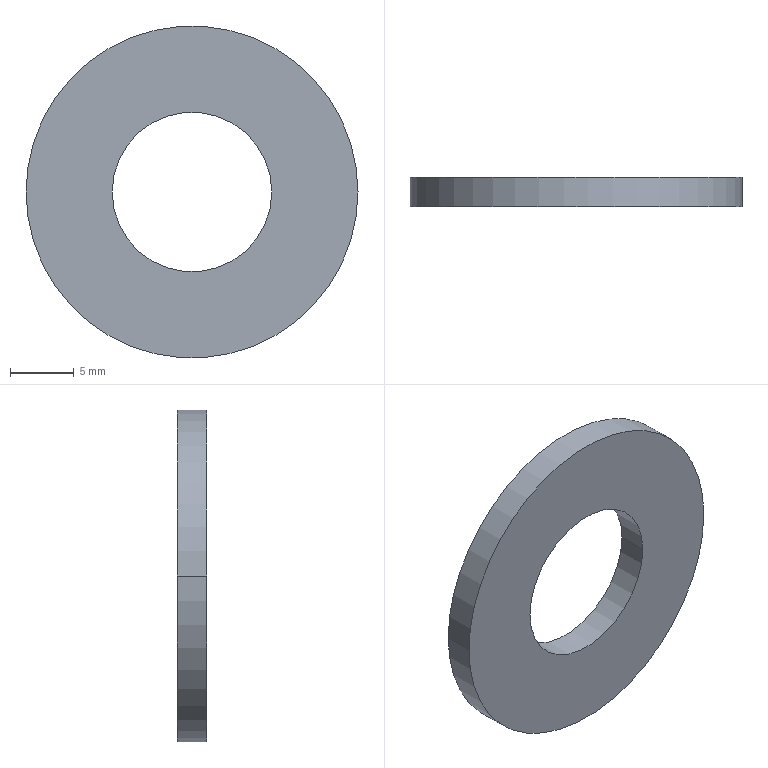Part | STEP file | ZZ21-M12 | 1 solid | 6 faces | box 26 x 2.3 x 26 mm | volume 938.885 mm3 | cylinder 4 | plane 2 | commonest cylinder face diameters 12.5 x2 26 x2
STEP:
#1=CARTESIAN_POINT('',(0.,0.,0.));
#2=DIRECTION('',(0.,0.,1.));
#3=DIRECTION('',(1.,0.,0.));
#4=AXIS2_PLACEMENT_3D('',#1,#2,#3);
#5=CARTESIAN_POINT('',(-6.25,0.,0.));
#6=VERTEX_POINT('',#5);
#7=CARTESIAN_POINT('',(-6.25,2.3,0.));
#8=VERTEX_POINT('',#7);
#9=CARTESIAN_POINT('',(-6.25,0.,0.));
#10=DIRECTION('',(0.,1.,0.));
#11=VECTOR('',#10,1.);
#12=LINE('',#9,#11);
#13=CARTESIAN_POINT('',(0.,0.,0.));
#14=DIRECTION('',(0.,1.,0.));
#15=DIRECTION('',(-1.,0.,0.));
#16=AXIS2_PLACEMENT_3D('',#13,#14,#15);
#17=CYLINDRICAL_SURFACE('',#16,6.25);
#18=CARTESIAN_POINT('',(6.283,0.));
#19=DIRECTION('',(0.,1.));
#20=VECTOR('',#19,1.);
#21=LINE('',#18,#20);
#22=(GEOMETRIC_REPRESENTATION_CONTEXT(2)PARAMETRIC_REPRESENTATION_CONTEXT()REPRESENTATION_CONTEXT('',''));
#23=DEFINITIONAL_REPRESENTATION('',(#21),#22);
#24=PCURVE('',#17,#23);
#25=CARTESIAN_POINT('',(0.,0.,0.));
#26=DIRECTION('',(0.,1.,0.));
#27=DIRECTION('',(-1.,0.,0.));
#28=AXIS2_PLACEMENT_3D('',#25,#26,#27);
#29=CYLINDRICAL_SURFACE('',#28,6.25);
#30=CARTESIAN_POINT('',(0.,0.));
#31=DIRECTION('',(0.,1.));
#32=VECTOR('',#31,1.);
#33=LINE('',#30,#32);
#34=(GEOMETRIC_REPRESENTATION_CONTEXT(2)PARAMETRIC_REPRESENTATION_CONTEXT()REPRESENTATION_CONTEXT('',''));
#35=DEFINITIONAL_REPRESENTATION('',(#33),#34);
#36=PCURVE('',#29,#35);
#37=SURFACE_CURVE('',#12,(#24,#36),.PCURVE_S1.);
#38=EDGE_CURVE('',#6,#8,#37,.T.);
#39=ORIENTED_EDGE('',*,*,#38,.T.);
#40=CARTESIAN_POINT('',(6.25,2.3,0.));
#41=VERTEX_POINT('',#40);
#42=CARTESIAN_POINT('',(0.,2.3,0.));
#43=DIRECTION('',(0.,-1.,0.));
#44=DIRECTION('',(1.,0.,0.));
#45=AXIS2_PLACEMENT_3D('',#42,#43,#44);
#46=CIRCLE('',#45,6.25);
#47=CARTESIAN_POINT('',(9.425,2.3));
#48=DIRECTION('',(-1.,0.));
#49=VECTOR('',#48,1.);
#50=LINE('',#47,#49);
#51=(GEOMETRIC_REPRESENTATION_CONTEXT(2)PARAMETRIC_REPRESENTATION_CONTEXT()REPRESENTATION_CONTEXT('',''));
#52=DEFINITIONAL_REPRESENTATION('',(#50),#51);
#53=PCURVE('',#17,#52);
#54=CARTESIAN_POINT('',(0.,2.3,0.));
#55=DIRECTION('',(0.,1.,0.));
#56=DIRECTION('',(-1.,0.,0.));
#57=AXIS2_PLACEMENT_3D('',#54,#55,#56);
#58=PLANE('',#57);
#59=CARTESIAN_POINT('',(-6.25,0.));
#60=CARTESIAN_POINT('',(-6.25,10.825));
#61=CARTESIAN_POINT('',(3.125,5.413));
#62=CARTESIAN_POINT('',(12.5,0.));
#63=CARTESIAN_POINT('',(3.125,-5.413));
#64=CARTESIAN_POINT('',(-6.25,-10.825));
#65=CARTESIAN_POINT('',(-6.25,0.));
#66=(BOUNDED_CURVE()B_SPLINE_CURVE(2,(#59,#60,#61,#62,#63,#64,#65),.UNSPECIFIED.,.T.,.F.)B_SPLINE_CURVE_WITH_KNOTS((1,2,2,2,2,1),(-2.094,0.,2.094,4.189,6.283,8.378),.UNSPECIFIED.)CURVE()GEOMETRIC_REPRESENTATION_ITEM()RATIONAL_B_SPLINE_CURVE((1.,0.5,1.,0.5,1.,0.5,1.))REPRESENTATION_ITEM(''));
#67=(GEOMETRIC_REPRESENTATION_CONTEXT(2)PARAMETRIC_REPRESENTATION_CONTEXT()REPRESENTATION_CONTEXT('',''));
#68=DEFINITIONAL_REPRESENTATION('',(#66),#67);
#69=PCURVE('',#58,#68);
#70=SURFACE_CURVE('',#46,(#53,#69),.PCURVE_S1.);
#71=EDGE_CURVE('',#8,#41,#70,.T.);
#72=ORIENTED_EDGE('',*,*,#71,.T.);
#73=CARTESIAN_POINT('',(6.25,0.,0.));
#74=VERTEX_POINT('',#73);
#75=CARTESIAN_POINT('',(6.25,0.,0.));
#76=DIRECTION('',(0.,1.,0.));
#77=VECTOR('',#76,1.);
#78=LINE('',#75,#77);
#79=CARTESIAN_POINT('',(3.142,0.));
#80=DIRECTION('',(0.,1.));
#81=VECTOR('',#80,1.);
#82=LINE('',#79,#81);
#83=(GEOMETRIC_REPRESENTATION_CONTEXT(2)PARAMETRIC_REPRESENTATION_CONTEXT()REPRESENTATION_CONTEXT('',''));
#84=DEFINITIONAL_REPRESENTATION('',(#82),#83);
#85=PCURVE('',#17,#84);
#86=CARTESIAN_POINT('',(3.142,0.));
#87=DIRECTION('',(0.,1.));
#88=VECTOR('',#87,1.);
#89=LINE('',#86,#88);
#90=(GEOMETRIC_REPRESENTATION_CONTEXT(2)PARAMETRIC_REPRESENTATION_CONTEXT()REPRESENTATION_CONTEXT('',''));
#91=DEFINITIONAL_REPRESENTATION('',(#89),#90);
#92=PCURVE('',#29,#91);
#93=SURFACE_CURVE('',#78,(#85,#92),.PCURVE_S1.);
#94=EDGE_CURVE('',#74,#41,#93,.T.);
#95=ORIENTED_EDGE('',*,*,#94,.F.);
#96=CARTESIAN_POINT('',(0.,0.,0.));
#97=DIRECTION('',(0.,1.,0.));
#98=DIRECTION('',(-1.,0.,0.));
#99=AXIS2_PLACEMENT_3D('',#96,#97,#98);
#100=CIRCLE('',#99,6.25);
#101=CARTESIAN_POINT('',(0.,0.));
#102=DIRECTION('',(1.,0.));
#103=VECTOR('',#102,1.);
#104=LINE('',#101,#103);
#105=(GEOMETRIC_REPRESENTATION_CONTEXT(2)PARAMETRIC_REPRESENTATION_CONTEXT()REPRESENTATION_CONTEXT('',''));
#106=DEFINITIONAL_REPRESENTATION('',(#104),#105);
#107=PCURVE('',#17,#106);
#108=CARTESIAN_POINT('',(0.,0.,0.));
#109=DIRECTION('',(0.,-1.,0.));
#110=DIRECTION('',(1.,0.,0.));
#111=AXIS2_PLACEMENT_3D('',#108,#109,#110);
#112=PLANE('',#111);
#113=CARTESIAN_POINT('',(-6.25,0.));
#114=CARTESIAN_POINT('',(-6.25,10.825));
#115=CARTESIAN_POINT('',(3.125,5.413));
#116=CARTESIAN_POINT('',(12.5,0.));
#117=CARTESIAN_POINT('',(3.125,-5.413));
#118=CARTESIAN_POINT('',(-6.25,-10.825));
#119=CARTESIAN_POINT('',(-6.25,0.));
#120=(BOUNDED_CURVE()B_SPLINE_CURVE(2,(#113,#114,#115,#116,#117,#118,#119),.UNSPECIFIED.,.T.,.F.)B_SPLINE_CURVE_WITH_KNOTS((1,2,2,2,2,1),(-2.094,0.,2.094,4.189,6.283,8.378),.UNSPECIFIED.)CURVE()GEOMETRIC_REPRESENTATION_ITEM()RATIONAL_B_SPLINE_CURVE((1.,0.5,1.,0.5,1.,0.5,1.))REPRESENTATION_ITEM(''));
#121=(GEOMETRIC_REPRESENTATION_CONTEXT(2)PARAMETRIC_REPRESENTATION_CONTEXT()REPRESENTATION_CONTEXT('',''));
#122=DEFINITIONAL_REPRESENTATION('',(#120),#121);
#123=PCURVE('',#112,#122);
#124=SURFACE_CURVE('',#100,(#107,#123),.PCURVE_S1.);
#125=EDGE_CURVE('',#74,#6,#124,.T.);
#126=ORIENTED_EDGE('',*,*,#125,.T.);
#127=EDGE_LOOP('',(#39,#72,#95,#126));
#128=FACE_BOUND('',#127,.F.);
#129=ADVANCED_FACE('',(#128),#17,.F.);
#130=CARTESIAN_POINT('',(-13.,0.,0.));
#131=VERTEX_POINT('',#130);
#132=CARTESIAN_POINT('',(13.,0.,0.));
#133=VERTEX_POINT('',#132);
#134=CARTESIAN_POINT('',(0.,0.,0.));
#135=DIRECTION('',(0.,1.,0.));
#136=DIRECTION('',(-1.,0.,0.));
#137=AXIS2_PLACEMENT_3D('',#134,#135,#136);
#138=CIRCLE('',#137,13.);
#139=CARTESIAN_POINT('',(0.,0.,0.));
#140=DIRECTION('',(0.,1.,0.));
#141=DIRECTION('',(-1.,0.,0.));
#142=AXIS2_PLACEMENT_3D('',#139,#140,#141);
#143=CYLINDRICAL_SURFACE('',#142,13.);
#144=CARTESIAN_POINT('',(0.,0.));
#145=DIRECTION('',(1.,0.));
#146=VECTOR('',#145,1.);
#147=LINE('',#144,#146);
#148=(GEOMETRIC_REPRESENTATION_CONTEXT(2)PARAMETRIC_REPRESENTATION_CONTEXT()REPRESENTATION_CONTEXT('',''));
#149=DEFINITIONAL_REPRESENTATION('',(#147),#148);
#150=PCURVE('',#143,#149);
#151=CARTESIAN_POINT('',(-13.,0.));
#152=CARTESIAN_POINT('',(-13.,22.517));
#153=CARTESIAN_POINT('',(6.5,11.258));
#154=CARTESIAN_POINT('',(26.,0.));
#155=CARTESIAN_POINT('',(6.5,-11.258));
#156=CARTESIAN_POINT('',(-13.,-22.517));
#157=CARTESIAN_POINT('',(-13.,0.));
#158=(BOUNDED_CURVE()B_SPLINE_CURVE(2,(#151,#152,#153,#154,#155,#156,#157),.UNSPECIFIED.,.T.,.F.)B_SPLINE_CURVE_WITH_KNOTS((1,2,2,2,2,1),(-2.094,0.,2.094,4.189,6.283,8.378),.UNSPECIFIED.)CURVE()GEOMETRIC_REPRESENTATION_ITEM()RATIONAL_B_SPLINE_CURVE((1.,0.5,1.,0.5,1.,0.5,1.))REPRESENTATION_ITEM(''));
#159=(GEOMETRIC_REPRESENTATION_CONTEXT(2)PARAMETRIC_REPRESENTATION_CONTEXT()REPRESENTATION_CONTEXT('',''));
#160=DEFINITIONAL_REPRESENTATION('',(#158),#159);
#161=PCURVE('',#112,#160);
#162=SURFACE_CURVE('',#138,(#150,#161),.PCURVE_S1.);
#163=EDGE_CURVE('',#131,#133,#162,.T.);
#164=ORIENTED_EDGE('',*,*,#163,.T.);
#165=CARTESIAN_POINT('',(13.,2.3,0.));
#166=VERTEX_POINT('',#165);
#167=CARTESIAN_POINT('',(13.,0.,0.));
#168=DIRECTION('',(0.,1.,0.));
#169=VECTOR('',#168,1.);
#170=LINE('',#167,#169);
#171=CARTESIAN_POINT('',(3.142,0.));
#172=DIRECTION('',(0.,1.));
#173=VECTOR('',#172,1.);
#174=LINE('',#171,#173);
#175=(GEOMETRIC_REPRESENTATION_CONTEXT(2)PARAMETRIC_REPRESENTATION_CONTEXT()REPRESENTATION_CONTEXT('',''));
#176=DEFINITIONAL_REPRESENTATION('',(#174),#175);
#177=PCURVE('',#143,#176);
#178=CARTESIAN_POINT('',(0.,0.,0.));
#179=DIRECTION('',(0.,1.,0.));
#180=DIRECTION('',(-1.,0.,0.));
#181=AXIS2_PLACEMENT_3D('',#178,#179,#180);
#182=CYLINDRICAL_SURFACE('',#181,13.);
#183=CARTESIAN_POINT('',(3.142,0.));
#184=DIRECTION('',(0.,1.));
#185=VECTOR('',#184,1.);
#186=LINE('',#183,#185);
#187=(GEOMETRIC_REPRESENTATION_CONTEXT(2)PARAMETRIC_REPRESENTATION_CONTEXT()REPRESENTATION_CONTEXT('',''));
#188=DEFINITIONAL_REPRESENTATION('',(#186),#187);
#189=PCURVE('',#182,#188);
#190=SURFACE_CURVE('',#170,(#177,#189),.PCURVE_S1.);
#191=EDGE_CURVE('',#133,#166,#190,.T.);
#192=ORIENTED_EDGE('',*,*,#191,.T.);
#193=CARTESIAN_POINT('',(-13.,2.3,0.));
#194=VERTEX_POINT('',#193);
#195=CARTESIAN_POINT('',(0.,2.3,0.));
#196=DIRECTION('',(0.,-1.,0.));
#197=DIRECTION('',(1.,0.,0.));
#198=AXIS2_PLACEMENT_3D('',#195,#196,#197);
#199=CIRCLE('',#198,13.);
#200=CARTESIAN_POINT('',(3.142,2.3));
#201=DIRECTION('',(-1.,0.));
#202=VECTOR('',#201,1.);
#203=LINE('',#200,#202);
#204=(GEOMETRIC_REPRESENTATION_CONTEXT(2)PARAMETRIC_REPRESENTATION_CONTEXT()REPRESENTATION_CONTEXT('',''));
#205=DEFINITIONAL_REPRESENTATION('',(#203),#204);
#206=PCURVE('',#143,#205);
#207=CARTESIAN_POINT('',(-13.,0.));
#208=CARTESIAN_POINT('',(-13.,22.517));
#209=CARTESIAN_POINT('',(6.5,11.258));
#210=CARTESIAN_POINT('',(26.,0.));
#211=CARTESIAN_POINT('',(6.5,-11.258));
#212=CARTESIAN_POINT('',(-13.,-22.517));
#213=CARTESIAN_POINT('',(-13.,0.));
#214=(BOUNDED_CURVE()B_SPLINE_CURVE(2,(#207,#208,#209,#210,#211,#212,#213),.UNSPECIFIED.,.T.,.F.)B_SPLINE_CURVE_WITH_KNOTS((1,2,2,2,2,1),(-2.094,0.,2.094,4.189,6.283,8.378),.UNSPECIFIED.)CURVE()GEOMETRIC_REPRESENTATION_ITEM()RATIONAL_B_SPLINE_CURVE((1.,0.5,1.,0.5,1.,0.5,1.))REPRESENTATION_ITEM(''));
#215=(GEOMETRIC_REPRESENTATION_CONTEXT(2)PARAMETRIC_REPRESENTATION_CONTEXT()REPRESENTATION_CONTEXT('',''));
#216=DEFINITIONAL_REPRESENTATION('',(#214),#215);
#217=PCURVE('',#58,#216);
#218=SURFACE_CURVE('',#199,(#206,#217),.PCURVE_S1.);
#219=EDGE_CURVE('',#166,#194,#218,.T.);
#220=ORIENTED_EDGE('',*,*,#219,.T.);
#221=CARTESIAN_POINT('',(-13.,0.,0.));
#222=DIRECTION('',(0.,1.,0.));
#223=VECTOR('',#222,1.);
#224=LINE('',#221,#223);
#225=CARTESIAN_POINT('',(0.,0.));
#226=DIRECTION('',(0.,1.));
#227=VECTOR('',#226,1.);
#228=LINE('',#225,#227);
#229=(GEOMETRIC_REPRESENTATION_CONTEXT(2)PARAMETRIC_REPRESENTATION_CONTEXT()REPRESENTATION_CONTEXT('',''));
#230=DEFINITIONAL_REPRESENTATION('',(#228),#229);
#231=PCURVE('',#143,#230);
#232=CARTESIAN_POINT('',(6.283,0.));
#233=DIRECTION('',(0.,1.));
#234=VECTOR('',#233,1.);
#235=LINE('',#232,#234);
#236=(GEOMETRIC_REPRESENTATION_CONTEXT(2)PARAMETRIC_REPRESENTATION_CONTEXT()REPRESENTATION_CONTEXT('',''));
#237=DEFINITIONAL_REPRESENTATION('',(#235),#236);
#238=PCURVE('',#182,#237);
#239=SURFACE_CURVE('',#224,(#231,#238),.PCURVE_S1.);
#240=EDGE_CURVE('',#131,#194,#239,.T.);
#241=ORIENTED_EDGE('',*,*,#240,.F.);
#242=EDGE_LOOP('',(#164,#192,#220,#241));
#243=FACE_BOUND('',#242,.T.);
#244=ADVANCED_FACE('',(#243),#143,.T.);
#245=ORIENTED_EDGE('',*,*,#71,.T.);
#246=CARTESIAN_POINT('',(0.,2.3,0.));
#247=DIRECTION('',(0.,-1.,0.));
#248=DIRECTION('',(1.,0.,0.));
#249=AXIS2_PLACEMENT_3D('',#246,#247,#248);
#250=CIRCLE('',#249,6.25);
#251=CARTESIAN_POINT('',(-6.25,0.));
#252=CARTESIAN_POINT('',(-6.25,10.825));
#253=CARTESIAN_POINT('',(3.125,5.413));
#254=CARTESIAN_POINT('',(12.5,0.));
#255=CARTESIAN_POINT('',(3.125,-5.413));
#256=CARTESIAN_POINT('',(-6.25,-10.825));
#257=CARTESIAN_POINT('',(-6.25,0.));
#258=(BOUNDED_CURVE()B_SPLINE_CURVE(2,(#251,#252,#253,#254,#255,#256,#257),.UNSPECIFIED.,.T.,.F.)B_SPLINE_CURVE_WITH_KNOTS((1,2,2,2,2,1),(-2.094,0.,2.094,4.189,6.283,8.378),.UNSPECIFIED.)CURVE()GEOMETRIC_REPRESENTATION_ITEM()RATIONAL_B_SPLINE_CURVE((1.,0.5,1.,0.5,1.,0.5,1.))REPRESENTATION_ITEM(''));
#259=(GEOMETRIC_REPRESENTATION_CONTEXT(2)PARAMETRIC_REPRESENTATION_CONTEXT()REPRESENTATION_CONTEXT('',''));
#260=DEFINITIONAL_REPRESENTATION('',(#258),#259);
#261=PCURVE('',#58,#260);
#262=CARTESIAN_POINT('',(3.142,2.3));
#263=DIRECTION('',(-1.,0.));
#264=VECTOR('',#263,1.);
#265=LINE('',#262,#264);
#266=(GEOMETRIC_REPRESENTATION_CONTEXT(2)PARAMETRIC_REPRESENTATION_CONTEXT()REPRESENTATION_CONTEXT('',''));
#267=DEFINITIONAL_REPRESENTATION('',(#265),#266);
#268=PCURVE('',#29,#267);
#269=SURFACE_CURVE('',#250,(#261,#268),.PCURVE_S1.);
#270=EDGE_CURVE('',#41,#8,#269,.T.);
#271=ORIENTED_EDGE('',*,*,#270,.T.);
#272=EDGE_LOOP('',(#245,#271));
#273=FACE_BOUND('',#272,.T.);
#274=CARTESIAN_POINT('',(0.,2.3,0.));
#275=DIRECTION('',(0.,-1.,0.));
#276=DIRECTION('',(1.,0.,0.));
#277=AXIS2_PLACEMENT_3D('',#274,#275,#276);
#278=CIRCLE('',#277,13.);
#279=CARTESIAN_POINT('',(-13.,0.));
#280=CARTESIAN_POINT('',(-13.,22.517));
#281=CARTESIAN_POINT('',(6.5,11.258));
#282=CARTESIAN_POINT('',(26.,0.));
#283=CARTESIAN_POINT('',(6.5,-11.258));
#284=CARTESIAN_POINT('',(-13.,-22.517));
#285=CARTESIAN_POINT('',(-13.,0.));
#286=(BOUNDED_CURVE()B_SPLINE_CURVE(2,(#279,#280,#281,#282,#283,#284,#285),.UNSPECIFIED.,.T.,.F.)B_SPLINE_CURVE_WITH_KNOTS((1,2,2,2,2,1),(-2.094,0.,2.094,4.189,6.283,8.378),.UNSPECIFIED.)CURVE()GEOMETRIC_REPRESENTATION_ITEM()RATIONAL_B_SPLINE_CURVE((1.,0.5,1.,0.5,1.,0.5,1.))REPRESENTATION_ITEM(''));
#287=(GEOMETRIC_REPRESENTATION_CONTEXT(2)PARAMETRIC_REPRESENTATION_CONTEXT()REPRESENTATION_CONTEXT('',''));
#288=DEFINITIONAL_REPRESENTATION('',(#286),#287);
#289=PCURVE('',#58,#288);
#290=CARTESIAN_POINT('',(9.425,2.3));
#291=DIRECTION('',(-1.,0.));
#292=VECTOR('',#291,1.);
#293=LINE('',#290,#292);
#294=(GEOMETRIC_REPRESENTATION_CONTEXT(2)PARAMETRIC_REPRESENTATION_CONTEXT()REPRESENTATION_CONTEXT('',''));
#295=DEFINITIONAL_REPRESENTATION('',(#293),#294);
#296=PCURVE('',#182,#295);
#297=SURFACE_CURVE('',#278,(#289,#296),.PCURVE_S1.);
#298=EDGE_CURVE('',#194,#166,#297,.T.);
#299=ORIENTED_EDGE('',*,*,#298,.F.);
#300=ORIENTED_EDGE('',*,*,#219,.F.);
#301=EDGE_LOOP('',(#299,#300));
#302=FACE_BOUND('',#301,.T.);
#303=ADVANCED_FACE('',(#273,#302),#58,.T.);
#304=CARTESIAN_POINT('',(0.,0.,0.));
#305=DIRECTION('',(0.,1.,0.));
#306=DIRECTION('',(-1.,0.,0.));
#307=AXIS2_PLACEMENT_3D('',#304,#305,#306);
#308=CIRCLE('',#307,6.25);
#309=CARTESIAN_POINT('',(-6.25,0.));
#310=CARTESIAN_POINT('',(-6.25,10.825));
#311=CARTESIAN_POINT('',(3.125,5.413));
#312=CARTESIAN_POINT('',(12.5,0.));
#313=CARTESIAN_POINT('',(3.125,-5.413));
#314=CARTESIAN_POINT('',(-6.25,-10.825));
#315=CARTESIAN_POINT('',(-6.25,0.));
#316=(BOUNDED_CURVE()B_SPLINE_CURVE(2,(#309,#310,#311,#312,#313,#314,#315),.UNSPECIFIED.,.T.,.F.)B_SPLINE_CURVE_WITH_KNOTS((1,2,2,2,2,1),(-2.094,0.,2.094,4.189,6.283,8.378),.UNSPECIFIED.)CURVE()GEOMETRIC_REPRESENTATION_ITEM()RATIONAL_B_SPLINE_CURVE((1.,0.5,1.,0.5,1.,0.5,1.))REPRESENTATION_ITEM(''));
#317=(GEOMETRIC_REPRESENTATION_CONTEXT(2)PARAMETRIC_REPRESENTATION_CONTEXT()REPRESENTATION_CONTEXT('',''));
#318=DEFINITIONAL_REPRESENTATION('',(#316),#317);
#319=PCURVE('',#112,#318);
#320=CARTESIAN_POINT('',(0.,0.));
#321=DIRECTION('',(1.,0.));
#322=VECTOR('',#321,1.);
#323=LINE('',#320,#322);
#324=(GEOMETRIC_REPRESENTATION_CONTEXT(2)PARAMETRIC_REPRESENTATION_CONTEXT()REPRESENTATION_CONTEXT('',''));
#325=DEFINITIONAL_REPRESENTATION('',(#323),#324);
#326=PCURVE('',#29,#325);
#327=SURFACE_CURVE('',#308,(#319,#326),.PCURVE_S1.);
#328=EDGE_CURVE('',#6,#74,#327,.T.);
#329=ORIENTED_EDGE('',*,*,#328,.T.);
#330=ORIENTED_EDGE('',*,*,#125,.T.);
#331=EDGE_LOOP('',(#329,#330));
#332=FACE_BOUND('',#331,.T.);
#333=ORIENTED_EDGE('',*,*,#163,.F.);
#334=CARTESIAN_POINT('',(0.,0.,0.));
#335=DIRECTION('',(0.,1.,0.));
#336=DIRECTION('',(-1.,0.,0.));
#337=AXIS2_PLACEMENT_3D('',#334,#335,#336);
#338=CIRCLE('',#337,13.);
#339=CARTESIAN_POINT('',(-13.,0.));
#340=CARTESIAN_POINT('',(-13.,22.517));
#341=CARTESIAN_POINT('',(6.5,11.258));
#342=CARTESIAN_POINT('',(26.,0.));
#343=CARTESIAN_POINT('',(6.5,-11.258));
#344=CARTESIAN_POINT('',(-13.,-22.517));
#345=CARTESIAN_POINT('',(-13.,0.));
#346=(BOUNDED_CURVE()B_SPLINE_CURVE(2,(#339,#340,#341,#342,#343,#344,#345),.UNSPECIFIED.,.T.,.F.)B_SPLINE_CURVE_WITH_KNOTS((1,2,2,2,2,1),(-2.094,0.,2.094,4.189,6.283,8.378),.UNSPECIFIED.)CURVE()GEOMETRIC_REPRESENTATION_ITEM()RATIONAL_B_SPLINE_CURVE((1.,0.5,1.,0.5,1.,0.5,1.))REPRESENTATION_ITEM(''));
#347=(GEOMETRIC_REPRESENTATION_CONTEXT(2)PARAMETRIC_REPRESENTATION_CONTEXT()REPRESENTATION_CONTEXT('',''));
#348=DEFINITIONAL_REPRESENTATION('',(#346),#347);
#349=PCURVE('',#112,#348);
#350=CARTESIAN_POINT('',(0.,0.));
#351=DIRECTION('',(1.,0.));
#352=VECTOR('',#351,1.);
#353=LINE('',#350,#352);
#354=(GEOMETRIC_REPRESENTATION_CONTEXT(2)PARAMETRIC_REPRESENTATION_CONTEXT()REPRESENTATION_CONTEXT('',''));
#355=DEFINITIONAL_REPRESENTATION('',(#353),#354);
#356=PCURVE('',#182,#355);
#357=SURFACE_CURVE('',#338,(#349,#356),.PCURVE_S1.);
#358=EDGE_CURVE('',#133,#131,#357,.T.);
#359=ORIENTED_EDGE('',*,*,#358,.F.);
#360=EDGE_LOOP('',(#333,#359));
#361=FACE_BOUND('',#360,.T.);
#362=ADVANCED_FACE('',(#332,#361),#112,.T.);
#363=ORIENTED_EDGE('',*,*,#191,.F.);
#364=ORIENTED_EDGE('',*,*,#358,.T.);
#365=ORIENTED_EDGE('',*,*,#240,.T.);
#366=ORIENTED_EDGE('',*,*,#298,.T.);
#367=EDGE_LOOP('',(#363,#364,#365,#366));
#368=FACE_BOUND('',#367,.T.);
#369=ADVANCED_FACE('',(#368),#182,.T.);
#370=ORIENTED_EDGE('',*,*,#270,.T.);
#371=ORIENTED_EDGE('',*,*,#38,.F.);
#372=ORIENTED_EDGE('',*,*,#328,.T.);
#373=ORIENTED_EDGE('',*,*,#94,.T.);
#374=EDGE_LOOP('',(#370,#371,#372,#373));
#375=FACE_BOUND('',#374,.F.);
#376=ADVANCED_FACE('',(#375),#29,.F.);
#377=CLOSED_SHELL('',(#129,#244,#303,#362,#369,#376));
#378=MANIFOLD_SOLID_BREP('',#377);
#379=(LENGTH_UNIT()NAMED_UNIT(*)SI_UNIT(.MILLI.,.METRE.));
#380=UNCERTAINTY_MEASURE_WITH_UNIT(LENGTH_MEASURE(0.0000001),#379,'','');
#381=(NAMED_UNIT(*)PLANE_ANGLE_UNIT()SI_UNIT($,.RADIAN.));
#382=(NAMED_UNIT(*)SI_UNIT($,.STERADIAN.)SOLID_ANGLE_UNIT());
#383=(GEOMETRIC_REPRESENTATION_CONTEXT(3)GLOBAL_UNCERTAINTY_ASSIGNED_CONTEXT((#380))GLOBAL_UNIT_ASSIGNED_CONTEXT((#379,#381,#382))REPRESENTATION_CONTEXT('',''));
#384=ADVANCED_BREP_SHAPE_REPRESENTATION('',(#4,#378),#383);